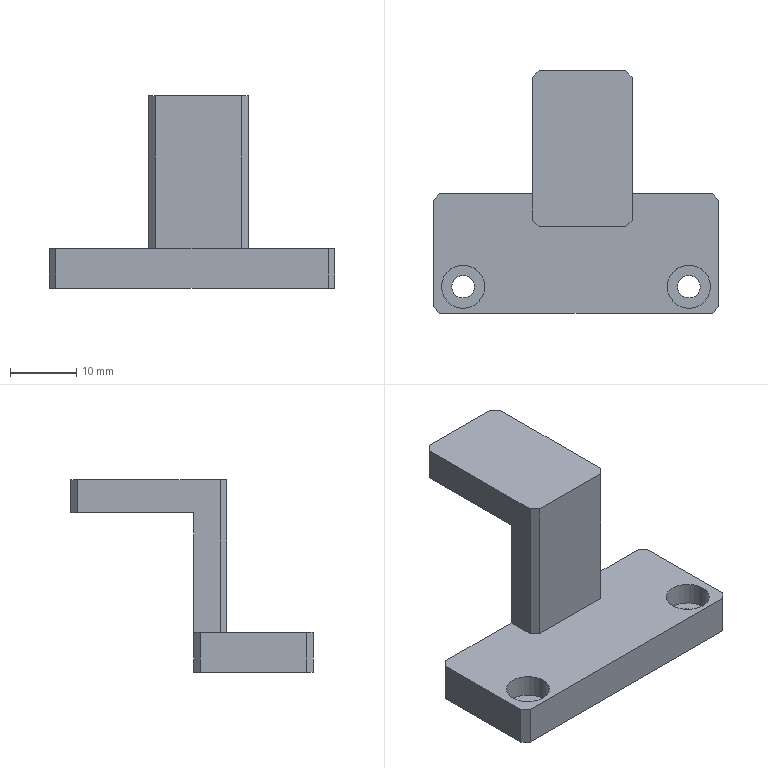CAM job | NX | 3-axis milling, drilling | part box 43 x 36.5 x 29 mm | stock box 48 x 40.5 x 35 mm
Tools:
number,name,description,diameter,corner_radius,flute_length,length,flutes
4,D4,平底铣刀-粗,4.0,0.0,25.0,75.0,2
9,D10,平底铣刀-粗,10.0,0.0,35.0,75.0,2
10,D10-J,平底铣刀-精,10.0,0.0,35.0,75.0,2
1,D80R0.8飞刀,圆鼻刀-粗,80.0,0.8,50.0,75.0,2
2,D6倒角刀,倒角刀,6.0,0.0,3.0,25.0,2
13,ZT3.4,钻头,3.4,0.0,35.0,50.0,2
Operations:
program,operation,operation_type,tool,method,geometry_group,spindle_rpm,surface_speed,feed_per_tooth,feed_cut,feed_plunge,cut_length_mm,path_length_mm,cut_time_min,machine_time_min
B,动态开粗D10_COPY_1,CavityMilling,D10,动态开粗-切深K-步距K,W-B,8000.0,251.32,0.25,4000.0,100.0,2802.092,2837.892,0.7005,0.7041
B,底壁铣分层开粗-中_COPY,VolumeBased25DMillingOperation,D10,分层开粗-切深K-步距G,W-B,8000.0,251.32,0.25,4000.0,100.0,14941.158,15029.141,3.735,3.744
B,铣沉头_1,CylinderMilling,D4,METHOD,W-B,6000.0,75.398,0.1,1200.0,100.0,296.666,508.866,0.2472,0.2684
B,铣孔_1,CylinderMilling,D4,METHOD,W-B,6000.0,75.398,0.05,600.0,100.0,22.642,242.242,0.0377,0.0597
B,平面去毛刺6X45L_COPY,SurfaceContour,D6倒角刀,爬面_倒角-切深0-步距G,W-B,6500.0,122.519,0.1154,1500.0,100.0,269.8,521.099,0.1799,0.205
B,底壁铣精光底面-中_COPY_2,VolumeBased25DMillingOperation,D10-J,精光步距切深关,W-B,7000.0,175.0,0.0536,1500.0,100.0,151.83,179.83,0.1012,0.104
B,底壁铣精光底面-中_COPY_1,VolumeBased25DMillingOperation,D10-J,精光步距切深关,W-B,7000.0,175.0,0.0536,1500.0,100.0,202.537,530.178,0.135,0.1678
B,底壁铣精光侧面-中-选底面_COPY,VolumeBased25DMillingOperation,D10-J,侧刃精光-切深K-步距G,W-B,8000.0,251.32,0.0625,1000.0,100.0,177.24,415.041,0.1772,0.201
A,顶面,FaceMilling,D80R0.8飞刀,侧刃精光-切深K-步距G,W-A,4000.0,1005.31,0.125,1000.0,100.0,137.0,173.0,0.137,0.1406
A,动态开粗D10_COPY,CavityMilling,D10,动态开粗-切深K-步距K,W-A,8000.0,251.32,0.25,4000.0,100.0,4495.001,4835.782,1.124,1.158
A,打点-深0.8,Operation,D6倒角刀,NONE,W-A,8000.0,150.796,0.0312,500.0,90.0,3.6,82.215,0.0072,0.0151
A,通孔-3-4,Operation,ZT3.4,NONE,W-A,3000.0,32.044,0.02,120.0,90.0,22.0,119.015,0.1833,0.193
A,仅选体,SurfaceContour,D6倒角刀,METHOD,W-A,8000.0,150.796,0.1875,3000.0,100.0,239.916,337.716,0.08,0.0898
A,钻倒角_1,Operation,D6倒角刀,METHOD,W-A,8000.0,150.796,0.0312,500.0,0.0,10.0,97.132,0.02,0.0287
A,底壁铣精光底面-中_COPY,VolumeBased25DMillingOperation,D10-J,精光步距切深关,W-A,7000.0,175.0,0.0536,1500.0,100.0,119.93,185.93,0.08,0.0866
A,等高精光-中_COPY,ZLevelMilling,D10-J,侧刃精光-切深K-步距G,W-A,8000.0,251.32,0.0625,1000.0,100.0,379.71,620.442,0.3797,0.4038